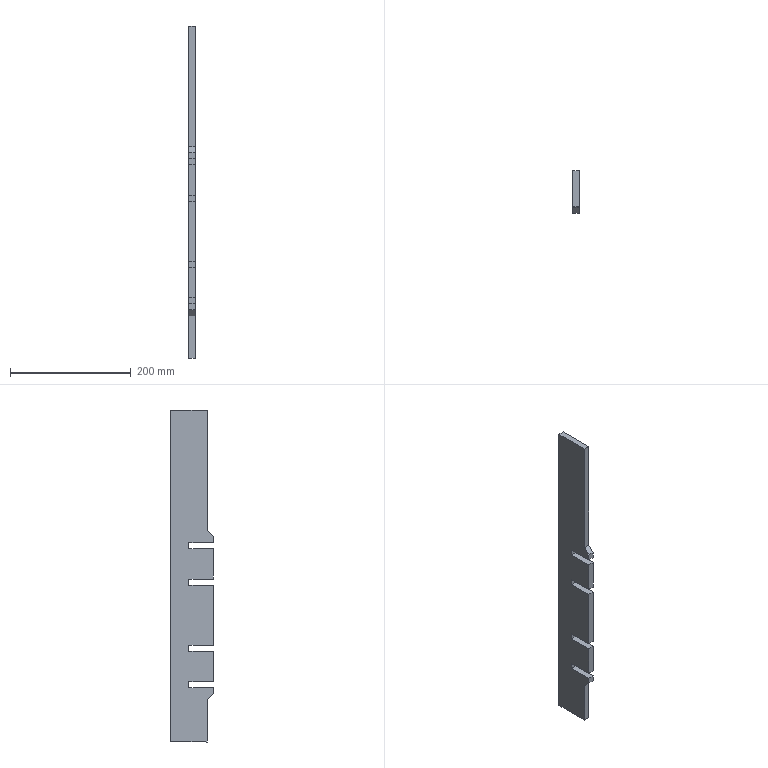Part | STEP file | subframe cylinder mounting plate reinforcement--000.001--202409
28 | 1 solid | 26 faces | box 10 x 70 x 550 mm | volume 341000 mm3 | plane 26